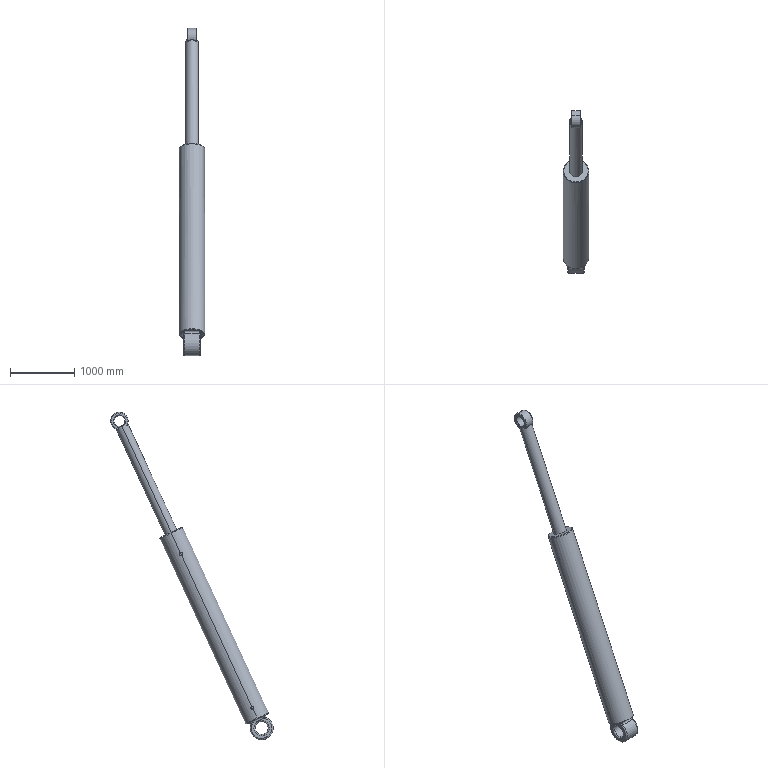Part | SolidWorks | 5 solids | 153 faces | box 400 x 2533 x 5104 mm | volume 258998356 mm3 | cylinder 52 | spline 40 | torus 33 | plane 26 | cone 2 | commonest cylinder face diameters 349 x8 200 x6 201 x6 20 x4 50 x4 60 x4